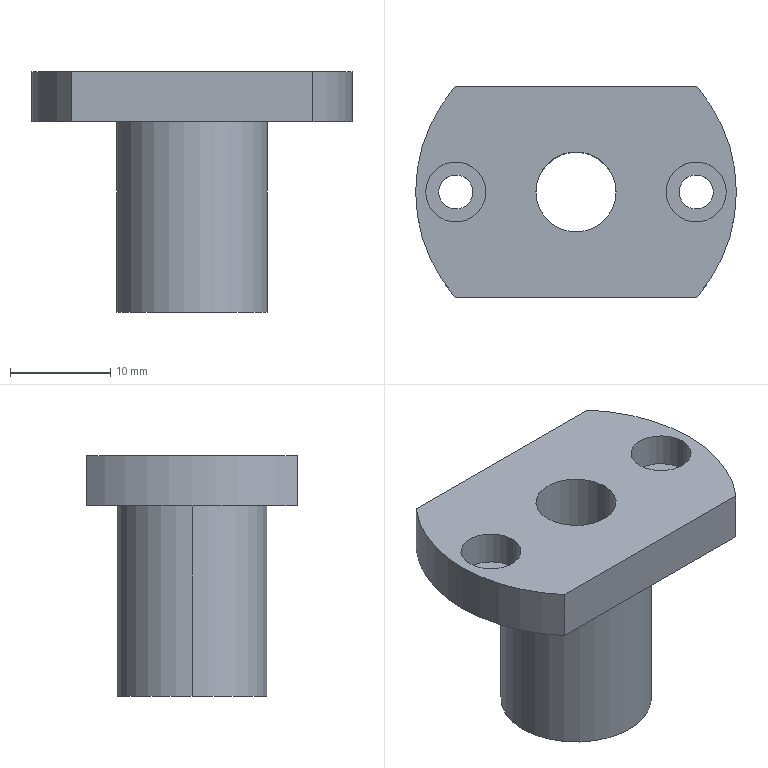Part | STEP file | LMH8UU | 1 solid | 22 faces | box 32 x 21 x 24 mm | volume 5030 mm3 | cylinder 15 | plane 7 | commonest cylinder face diameters 3.4 x4 6 x4 32 x3 8 x2 15 x2